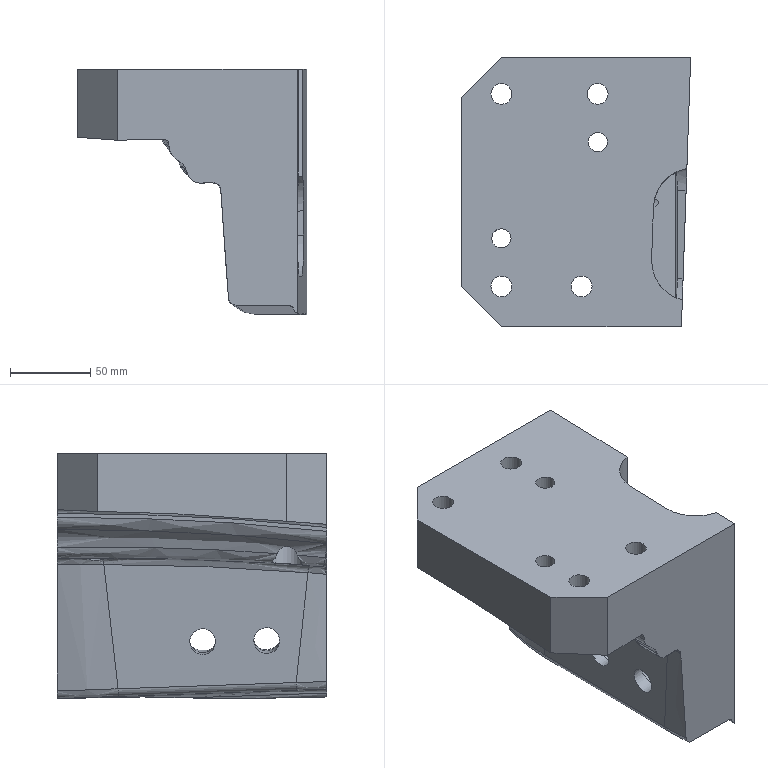Part | NX | features solid 2 | 1 solid | 66 faces | box 142.994 x 168.002 x 153.184 mm | volume 1617603 mm3 | spline 28 | cylinder 20 | plane 18 | commonest cylinder face diameters 20 x6 50 x6 13 x4 12 x2 16 x2